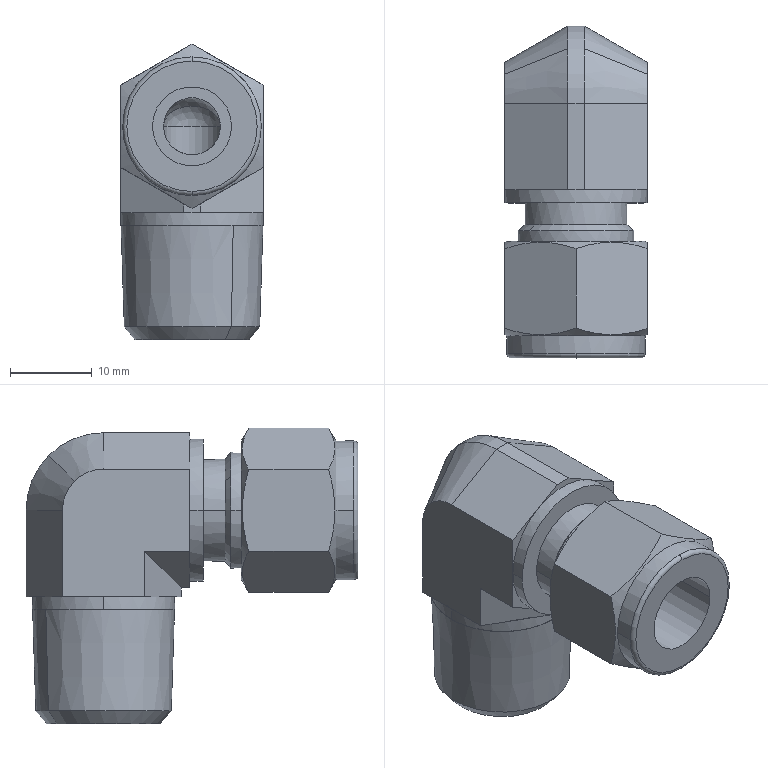Part | STEP file | FITTING-ELBOW-10A | 1 solid | 73 faces | box 17.46 x 40.703 x 36.281 mm | volume 10729 mm3 | plane 38 | cylinder 17 | cone 14 | sphere 2 | torus 2 | commonest cylinder face diameters 7 x4 17.46 x4 9.7 x2 12.5 x2 14.2 x2 17 x2